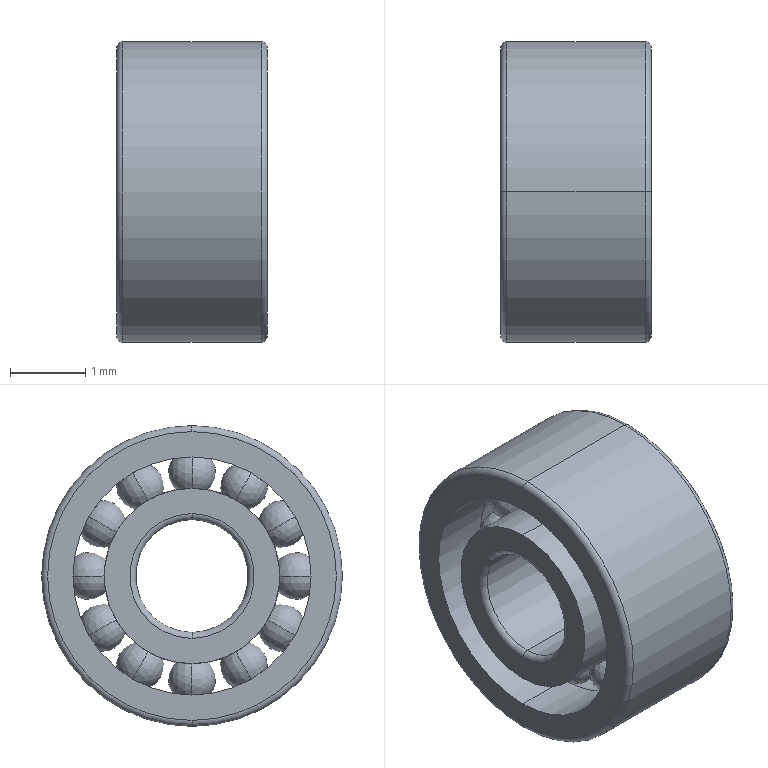Part | SolidWorks | features MoveCopyBody 1, Stock 1 | 1 solid | 84 faces | box 2 x 4 x 4 mm | volume 15.38 mm3 | torus 44 | sphere 24 | cylinder 12 | plane 4 | commonest cylinder face diameters 2.333 x4 3.167 x4 1.5 x2 4 x2